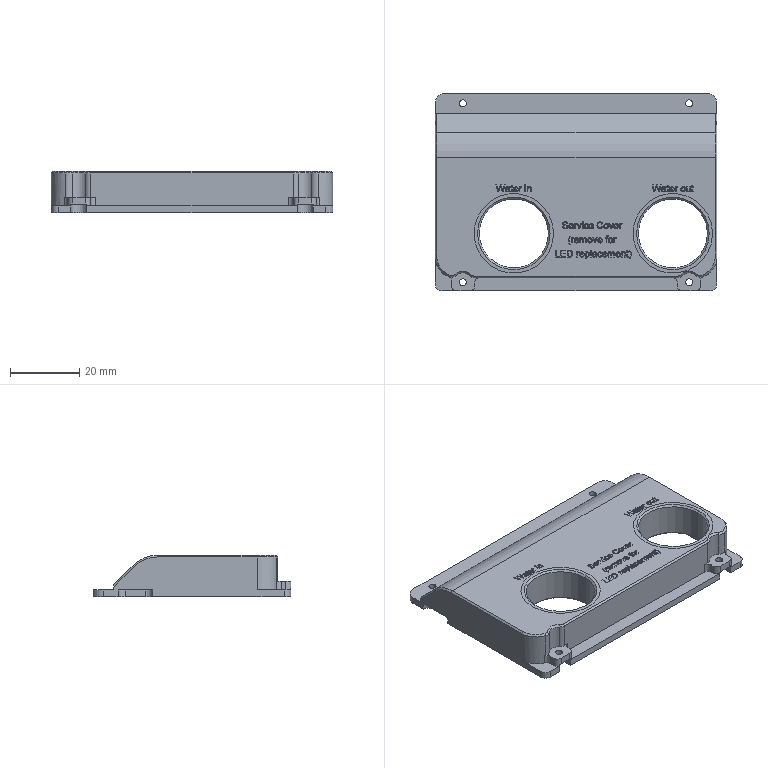Part | 2 solids | 1786 faces | box 81.5 x 57.25 x 12.01 mm | volume 41157 mm3 | plane 886 | cylinder 512 | spline 352 | cone 36 | commonest cylinder face diameters 4 x46 3 x24 0.751 x20 0.771 x20 0.817 x20 10.735 x20